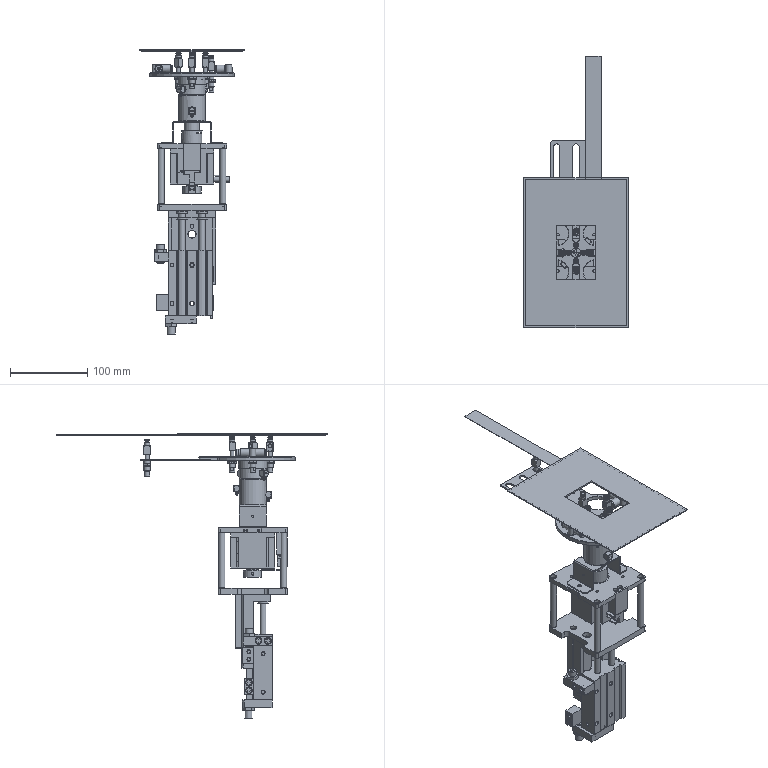Part | NX | 49 solids | 1889 faces | box 135 x 352.5 x 368.3 mm | volume 733827 mm3 | plane 940 | cylinder 512 | cone 370 | spline 42 | torus 25 | commonest cylinder face diameters 7 x43 2.5 x38 8 x31 10 x29 4.134 x23 4 x22